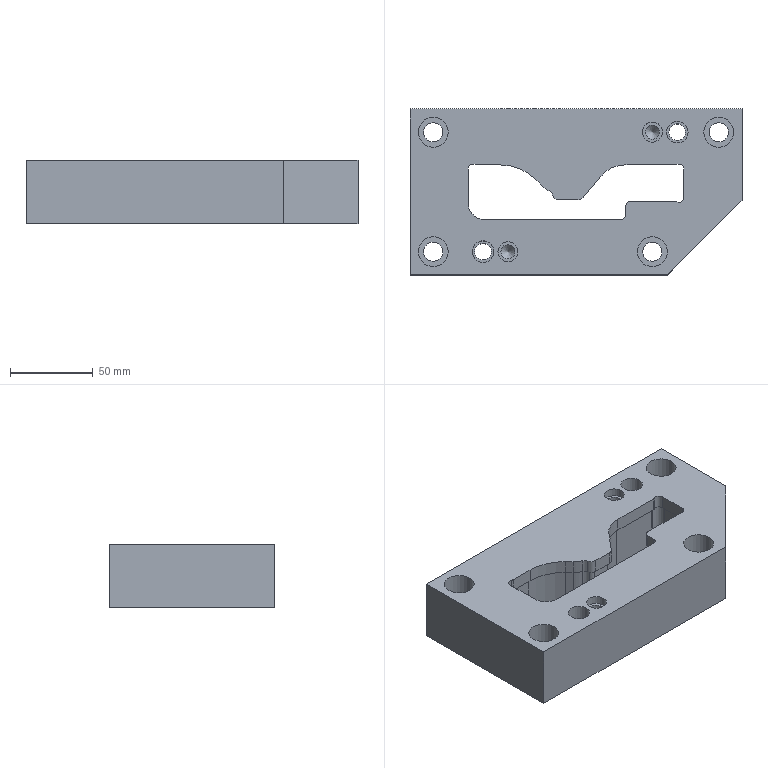Part | STEP file | lll_id206_x_t | 1 solid | 84 faces | box 200 x 100 x 38 mm | volume 548151 mm3 | cylinder 46 | plane 36 | cone 2 | commonest cylinder face diameters 6 x8 3 x4 9 x4 11.509 x4 18.008 x4 8 x3